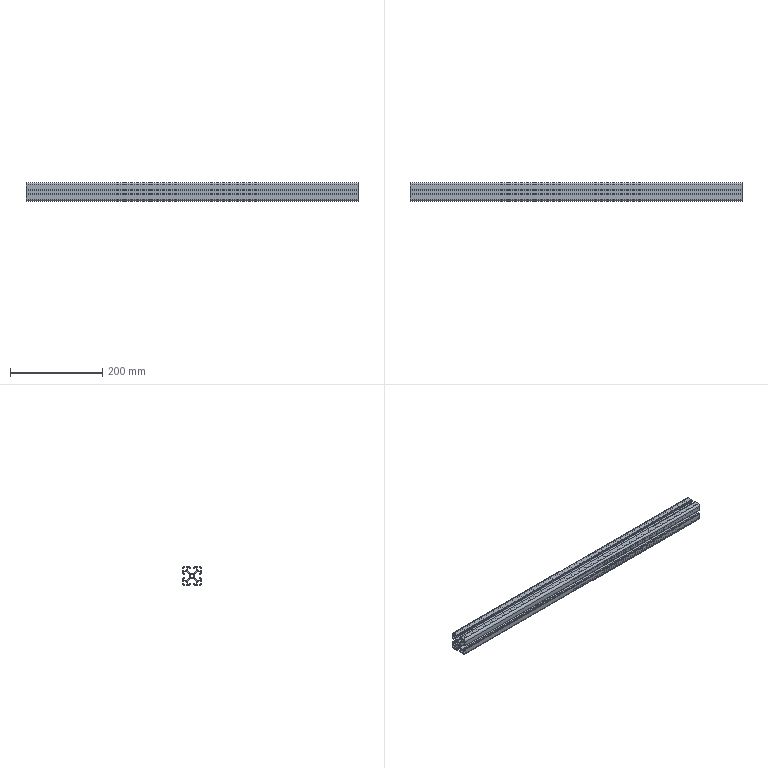Part | STEP file | MK-8-4040C-L-00 profile 4040C standard type 720mm | 1 solid | 188 faces | box 720 x 40 x 40 mm | volume 344339 mm3 | cylinder 94 | plane 94 | commonest cylinder face diameters 0.6 x30 2 x28 4 x16 0.4 x8 6 x4 9 x4